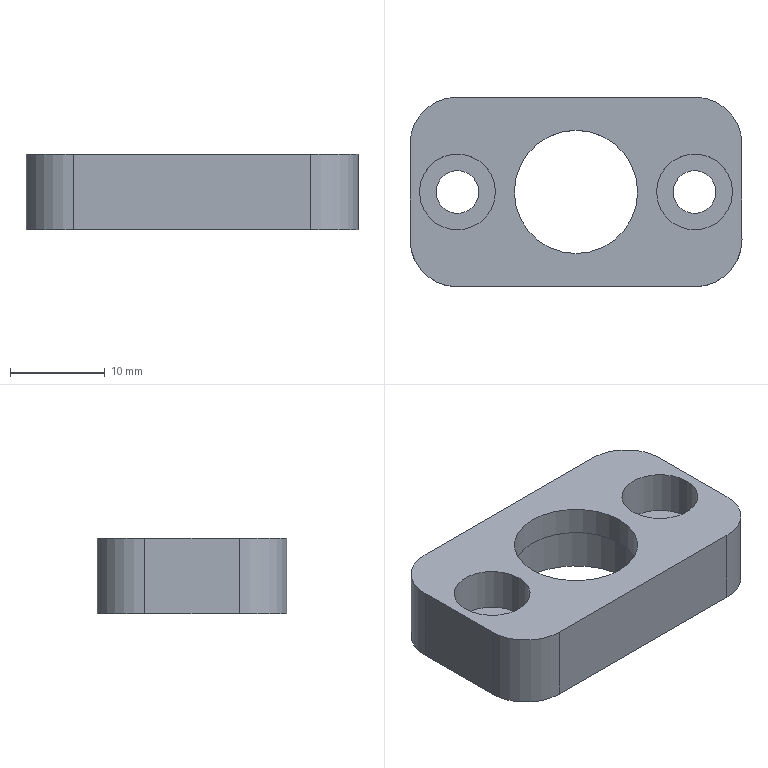Part | NX | 1 solid | 19 faces | box 35 x 20 x 8 mm | volume 3576 mm3 | cylinder 10 | plane 9 | commonest cylinder face diameters 10 x4 4.5 x2 8 x2 13 x1 15 x1
STEP:
#1=CARTESIAN_POINT('',(6.5,0.,8.));
#2=VERTEX_POINT('',#1);
#3=CARTESIAN_POINT('',(0.,0.,8.));
#4=DIRECTION('',(0.,0.,1.));
#5=DIRECTION('',(1.,0.,0.));
#6=AXIS2_PLACEMENT_3D('',#3,#4,#5);
#7=CIRCLE('',#6,6.5);
#8=EDGE_CURVE('',#2,#2,#7,.T.);
#9=ORIENTED_EDGE('',*,*,#8,.T.);
#10=EDGE_LOOP('',(#9));
#11=FACE_BOUND('',#10,.T.);
#12=CARTESIAN_POINT('',(-6.5,0.,5.));
#13=VERTEX_POINT('',#12);
#14=CARTESIAN_POINT('',(0.,0.,5.));
#15=DIRECTION('',(0.,0.,-1.));
#16=DIRECTION('',(-1.,0.,0.));
#17=AXIS2_PLACEMENT_3D('',#14,#15,#16);
#18=CIRCLE('',#17,6.5);
#19=EDGE_CURVE('',#13,#13,#18,.F.);
#20=ORIENTED_EDGE('',*,*,#19,.F.);
#21=EDGE_LOOP('',(#20));
#22=FACE_BOUND('',#21,.T.);
#23=CARTESIAN_POINT('',(0.,0.,0.));
#24=DIRECTION('',(0.,0.,1.));
#25=DIRECTION('',(1.,0.,0.));
#26=AXIS2_PLACEMENT_3D('',#23,#24,#25);
#27=CYLINDRICAL_SURFACE('',#26,6.5);
#28=ADVANCED_FACE('',(#11,#22),#27,.F.);
#29=CARTESIAN_POINT('',(17.5,-5.,8.));
#30=VERTEX_POINT('',#29);
#31=CARTESIAN_POINT('',(17.5,5.,8.));
#32=VERTEX_POINT('',#31);
#33=CARTESIAN_POINT('',(17.5,10.,8.));
#34=DIRECTION('',(0.,1.,0.));
#35=VECTOR('',#34,1000.);
#36=LINE('',#33,#35);
#37=EDGE_CURVE('',#30,#32,#36,.T.);
#38=ORIENTED_EDGE('',*,*,#37,.F.);
#39=CARTESIAN_POINT('',(17.5,-5.,0.));
#40=VERTEX_POINT('',#39);
#41=CARTESIAN_POINT('',(17.5,-5.,8.));
#42=DIRECTION('',(0.,0.,-1.));
#43=VECTOR('',#42,1000.);
#44=LINE('',#41,#43);
#45=EDGE_CURVE('',#30,#40,#44,.T.);
#46=ORIENTED_EDGE('',*,*,#45,.T.);
#47=CARTESIAN_POINT('',(17.5,5.,0.));
#48=VERTEX_POINT('',#47);
#49=CARTESIAN_POINT('',(17.5,10.,0.));
#50=DIRECTION('',(0.,1.,0.));
#51=VECTOR('',#50,1000.);
#52=LINE('',#49,#51);
#53=EDGE_CURVE('',#40,#48,#52,.T.);
#54=ORIENTED_EDGE('',*,*,#53,.T.);
#55=CARTESIAN_POINT('',(17.5,5.,8.));
#56=DIRECTION('',(0.,0.,-1.));
#57=VECTOR('',#56,1000.);
#58=LINE('',#55,#57);
#59=EDGE_CURVE('',#48,#32,#58,.F.);
#60=ORIENTED_EDGE('',*,*,#59,.T.);
#61=EDGE_LOOP('',(#38,#46,#54,#60));
#62=FACE_BOUND('',#61,.T.);
#63=CARTESIAN_POINT('',(17.5,10.,8.));
#64=DIRECTION('',(-1.,0.,0.));
#65=DIRECTION('',(0.,-1.,0.));
#66=AXIS2_PLACEMENT_3D('',#63,#64,#65);
#67=PLANE('',#66);
#68=ADVANCED_FACE('',(#62),#67,.F.);
#69=CARTESIAN_POINT('',(12.5,10.,0.));
#70=VERTEX_POINT('',#69);
#71=CARTESIAN_POINT('',(-12.5,10.,0.));
#72=VERTEX_POINT('',#71);
#73=CARTESIAN_POINT('',(-17.5,10.,0.));
#74=DIRECTION('',(-1.,0.,0.));
#75=VECTOR('',#74,1000.);
#76=LINE('',#73,#75);
#77=EDGE_CURVE('',#70,#72,#76,.T.);
#78=ORIENTED_EDGE('',*,*,#77,.T.);
#79=CARTESIAN_POINT('',(-12.5,10.,8.));
#80=VERTEX_POINT('',#79);
#81=CARTESIAN_POINT('',(-12.5,10.,8.));
#82=DIRECTION('',(0.,0.,-1.));
#83=VECTOR('',#82,1000.);
#84=LINE('',#81,#83);
#85=EDGE_CURVE('',#72,#80,#84,.F.);
#86=ORIENTED_EDGE('',*,*,#85,.T.);
#87=CARTESIAN_POINT('',(12.5,10.,8.));
#88=VERTEX_POINT('',#87);
#89=CARTESIAN_POINT('',(-17.5,10.,8.));
#90=DIRECTION('',(-1.,0.,0.));
#91=VECTOR('',#90,1000.);
#92=LINE('',#89,#91);
#93=EDGE_CURVE('',#88,#80,#92,.T.);
#94=ORIENTED_EDGE('',*,*,#93,.F.);
#95=CARTESIAN_POINT('',(12.5,10.,8.));
#96=DIRECTION('',(0.,0.,-1.));
#97=VECTOR('',#96,1000.);
#98=LINE('',#95,#97);
#99=EDGE_CURVE('',#88,#70,#98,.T.);
#100=ORIENTED_EDGE('',*,*,#99,.T.);
#101=EDGE_LOOP('',(#78,#86,#94,#100));
#102=FACE_BOUND('',#101,.T.);
#103=CARTESIAN_POINT('',(-17.5,10.,8.));
#104=DIRECTION('',(0.,-1.,0.));
#105=DIRECTION('',(0.,0.,-1.));
#106=AXIS2_PLACEMENT_3D('',#103,#104,#105);
#107=PLANE('',#106);
#108=ADVANCED_FACE('',(#102),#107,.F.);
#109=CARTESIAN_POINT('',(-17.5,5.,0.));
#110=VERTEX_POINT('',#109);
#111=CARTESIAN_POINT('',(-17.5,-5.,0.));
#112=VERTEX_POINT('',#111);
#113=CARTESIAN_POINT('',(-17.5,10.,0.));
#114=DIRECTION('',(0.,-1.,0.));
#115=VECTOR('',#114,1000.);
#116=LINE('',#113,#115);
#117=EDGE_CURVE('',#110,#112,#116,.T.);
#118=ORIENTED_EDGE('',*,*,#117,.T.);
#119=CARTESIAN_POINT('',(-17.5,-5.,8.));
#120=VERTEX_POINT('',#119);
#121=CARTESIAN_POINT('',(-17.5,-5.,8.));
#122=DIRECTION('',(0.,0.,-1.));
#123=VECTOR('',#122,1000.);
#124=LINE('',#121,#123);
#125=EDGE_CURVE('',#112,#120,#124,.F.);
#126=ORIENTED_EDGE('',*,*,#125,.T.);
#127=CARTESIAN_POINT('',(-17.5,5.,8.));
#128=VERTEX_POINT('',#127);
#129=CARTESIAN_POINT('',(-17.5,10.,8.));
#130=DIRECTION('',(0.,-1.,0.));
#131=VECTOR('',#130,1000.);
#132=LINE('',#129,#131);
#133=EDGE_CURVE('',#128,#120,#132,.T.);
#134=ORIENTED_EDGE('',*,*,#133,.F.);
#135=CARTESIAN_POINT('',(-17.5,5.,8.));
#136=DIRECTION('',(0.,0.,-1.));
#137=VECTOR('',#136,1000.);
#138=LINE('',#135,#137);
#139=EDGE_CURVE('',#128,#110,#138,.T.);
#140=ORIENTED_EDGE('',*,*,#139,.T.);
#141=EDGE_LOOP('',(#118,#126,#134,#140));
#142=FACE_BOUND('',#141,.T.);
#143=CARTESIAN_POINT('',(-17.5,10.,8.));
#144=DIRECTION('',(1.,0.,0.));
#145=DIRECTION('',(0.,1.,0.));
#146=AXIS2_PLACEMENT_3D('',#143,#144,#145);
#147=PLANE('',#146);
#148=ADVANCED_FACE('',(#142),#147,.F.);
#149=CARTESIAN_POINT('',(-12.5,-10.,0.));
#150=VERTEX_POINT('',#149);
#151=CARTESIAN_POINT('',(12.5,-10.,0.));
#152=VERTEX_POINT('',#151);
#153=CARTESIAN_POINT('',(-17.5,-10.,0.));
#154=DIRECTION('',(1.,0.,0.));
#155=VECTOR('',#154,1000.);
#156=LINE('',#153,#155);
#157=EDGE_CURVE('',#150,#152,#156,.T.);
#158=ORIENTED_EDGE('',*,*,#157,.T.);
#159=CARTESIAN_POINT('',(12.5,-10.,8.));
#160=VERTEX_POINT('',#159);
#161=CARTESIAN_POINT('',(12.5,-10.,8.));
#162=DIRECTION('',(0.,0.,-1.));
#163=VECTOR('',#162,1000.);
#164=LINE('',#161,#163);
#165=EDGE_CURVE('',#152,#160,#164,.F.);
#166=ORIENTED_EDGE('',*,*,#165,.T.);
#167=CARTESIAN_POINT('',(-12.5,-10.,8.));
#168=VERTEX_POINT('',#167);
#169=CARTESIAN_POINT('',(-17.5,-10.,8.));
#170=DIRECTION('',(1.,0.,0.));
#171=VECTOR('',#170,1000.);
#172=LINE('',#169,#171);
#173=EDGE_CURVE('',#168,#160,#172,.T.);
#174=ORIENTED_EDGE('',*,*,#173,.F.);
#175=CARTESIAN_POINT('',(-12.5,-10.,8.));
#176=DIRECTION('',(0.,0.,-1.));
#177=VECTOR('',#176,1000.);
#178=LINE('',#175,#177);
#179=EDGE_CURVE('',#168,#150,#178,.T.);
#180=ORIENTED_EDGE('',*,*,#179,.T.);
#181=EDGE_LOOP('',(#158,#166,#174,#180));
#182=FACE_BOUND('',#181,.T.);
#183=CARTESIAN_POINT('',(-17.5,-10.,8.));
#184=DIRECTION('',(0.,1.,0.));
#185=DIRECTION('',(0.,0.,1.));
#186=AXIS2_PLACEMENT_3D('',#183,#184,#185);
#187=PLANE('',#186);
#188=ADVANCED_FACE('',(#182),#187,.F.);
#189=CARTESIAN_POINT('',(-8.5,0.,8.));
#190=VERTEX_POINT('',#189);
#191=CARTESIAN_POINT('',(-12.5,0.,8.));
#192=DIRECTION('',(0.,0.,1.));
#193=DIRECTION('',(1.,0.,0.));
#194=AXIS2_PLACEMENT_3D('',#191,#192,#193);
#195=CIRCLE('',#194,4.);
#196=EDGE_CURVE('',#190,#190,#195,.T.);
#197=ORIENTED_EDGE('',*,*,#196,.F.);
#198=EDGE_LOOP('',(#197));
#199=FACE_BOUND('',#198,.T.);
#200=CARTESIAN_POINT('',(16.5,0.,8.));
#201=VERTEX_POINT('',#200);
#202=CARTESIAN_POINT('',(12.5,0.,8.));
#203=DIRECTION('',(0.,0.,1.));
#204=DIRECTION('',(1.,0.,0.));
#205=AXIS2_PLACEMENT_3D('',#202,#203,#204);
#206=CIRCLE('',#205,4.);
#207=EDGE_CURVE('',#201,#201,#206,.T.);
#208=ORIENTED_EDGE('',*,*,#207,.F.);
#209=EDGE_LOOP('',(#208));
#210=FACE_BOUND('',#209,.T.);
#211=ORIENTED_EDGE('',*,*,#8,.F.);
#212=EDGE_LOOP('',(#211));
#213=FACE_BOUND('',#212,.T.);
#214=ORIENTED_EDGE('',*,*,#173,.T.);
#215=CARTESIAN_POINT('',(12.5,-5.,8.));
#216=DIRECTION('',(0.,0.,1.));
#217=DIRECTION('',(1.,0.,0.));
#218=AXIS2_PLACEMENT_3D('',#215,#216,#217);
#219=CIRCLE('',#218,5.);
#220=EDGE_CURVE('',#160,#30,#219,.T.);
#221=ORIENTED_EDGE('',*,*,#220,.T.);
#222=ORIENTED_EDGE('',*,*,#37,.T.);
#223=CARTESIAN_POINT('',(12.5,5.,8.));
#224=DIRECTION('',(0.,0.,1.));
#225=DIRECTION('',(1.,0.,0.));
#226=AXIS2_PLACEMENT_3D('',#223,#224,#225);
#227=CIRCLE('',#226,5.);
#228=EDGE_CURVE('',#32,#88,#227,.T.);
#229=ORIENTED_EDGE('',*,*,#228,.T.);
#230=ORIENTED_EDGE('',*,*,#93,.T.);
#231=CARTESIAN_POINT('',(-12.5,5.,8.));
#232=DIRECTION('',(0.,0.,1.));
#233=DIRECTION('',(1.,0.,0.));
#234=AXIS2_PLACEMENT_3D('',#231,#232,#233);
#235=CIRCLE('',#234,5.);
#236=EDGE_CURVE('',#80,#128,#235,.T.);
#237=ORIENTED_EDGE('',*,*,#236,.T.);
#238=ORIENTED_EDGE('',*,*,#133,.T.);
#239=CARTESIAN_POINT('',(-12.5,-5.,8.));
#240=DIRECTION('',(0.,0.,1.));
#241=DIRECTION('',(1.,0.,0.));
#242=AXIS2_PLACEMENT_3D('',#239,#240,#241);
#243=CIRCLE('',#242,5.);
#244=EDGE_CURVE('',#120,#168,#243,.T.);
#245=ORIENTED_EDGE('',*,*,#244,.T.);
#246=EDGE_LOOP('',(#214,#221,#222,#229,#230,#237,#238,#245));
#247=FACE_BOUND('',#246,.T.);
#248=CARTESIAN_POINT('',(0.,0.,8.));
#249=DIRECTION('',(0.,0.,1.));
#250=DIRECTION('',(1.,0.,0.));
#251=AXIS2_PLACEMENT_3D('',#248,#249,#250);
#252=PLANE('',#251);
#253=ADVANCED_FACE('',(#199,#210,#213,#247),#252,.T.);
#254=CARTESIAN_POINT('',(-7.5,0.,0.));
#255=VERTEX_POINT('',#254);
#256=CARTESIAN_POINT('',(0.,0.,0.));
#257=DIRECTION('',(0.,0.,-1.));
#258=DIRECTION('',(-1.,0.,0.));
#259=AXIS2_PLACEMENT_3D('',#256,#257,#258);
#260=CIRCLE('',#259,7.5);
#261=EDGE_CURVE('',#255,#255,#260,.T.);
#262=ORIENTED_EDGE('',*,*,#261,.F.);
#263=EDGE_LOOP('',(#262));
#264=FACE_BOUND('',#263,.T.);
#265=CARTESIAN_POINT('',(-10.25,0.,0.));
#266=VERTEX_POINT('',#265);
#267=CARTESIAN_POINT('',(-12.5,0.,0.));
#268=DIRECTION('',(0.,0.,1.));
#269=DIRECTION('',(1.,0.,0.));
#270=AXIS2_PLACEMENT_3D('',#267,#268,#269);
#271=CIRCLE('',#270,2.25);
#272=EDGE_CURVE('',#266,#266,#271,.T.);
#273=ORIENTED_EDGE('',*,*,#272,.T.);
#274=EDGE_LOOP('',(#273));
#275=FACE_BOUND('',#274,.T.);
#276=CARTESIAN_POINT('',(14.75,0.,0.));
#277=VERTEX_POINT('',#276);
#278=CARTESIAN_POINT('',(12.5,0.,0.));
#279=DIRECTION('',(0.,0.,1.));
#280=DIRECTION('',(1.,0.,0.));
#281=AXIS2_PLACEMENT_3D('',#278,#279,#280);
#282=CIRCLE('',#281,2.25);
#283=EDGE_CURVE('',#277,#277,#282,.T.);
#284=ORIENTED_EDGE('',*,*,#283,.T.);
#285=EDGE_LOOP('',(#284));
#286=FACE_BOUND('',#285,.T.);
#287=ORIENTED_EDGE('',*,*,#53,.F.);
#288=CARTESIAN_POINT('',(12.5,-5.,0.));
#289=DIRECTION('',(0.,0.,1.));
#290=DIRECTION('',(1.,0.,0.));
#291=AXIS2_PLACEMENT_3D('',#288,#289,#290);
#292=CIRCLE('',#291,5.);
#293=EDGE_CURVE('',#40,#152,#292,.F.);
#294=ORIENTED_EDGE('',*,*,#293,.T.);
#295=ORIENTED_EDGE('',*,*,#157,.F.);
#296=CARTESIAN_POINT('',(-12.5,-5.,0.));
#297=DIRECTION('',(0.,0.,1.));
#298=DIRECTION('',(1.,0.,0.));
#299=AXIS2_PLACEMENT_3D('',#296,#297,#298);
#300=CIRCLE('',#299,5.);
#301=EDGE_CURVE('',#150,#112,#300,.F.);
#302=ORIENTED_EDGE('',*,*,#301,.T.);
#303=ORIENTED_EDGE('',*,*,#117,.F.);
#304=CARTESIAN_POINT('',(-12.5,5.,0.));
#305=DIRECTION('',(0.,0.,1.));
#306=DIRECTION('',(1.,0.,0.));
#307=AXIS2_PLACEMENT_3D('',#304,#305,#306);
#308=CIRCLE('',#307,5.);
#309=EDGE_CURVE('',#110,#72,#308,.F.);
#310=ORIENTED_EDGE('',*,*,#309,.T.);
#311=ORIENTED_EDGE('',*,*,#77,.F.);
#312=CARTESIAN_POINT('',(12.5,5.,0.));
#313=DIRECTION('',(0.,0.,1.));
#314=DIRECTION('',(1.,0.,0.));
#315=AXIS2_PLACEMENT_3D('',#312,#313,#314);
#316=CIRCLE('',#315,5.);
#317=EDGE_CURVE('',#70,#48,#316,.F.);
#318=ORIENTED_EDGE('',*,*,#317,.T.);
#319=EDGE_LOOP('',(#287,#294,#295,#302,#303,#310,#311,#318));
#320=FACE_BOUND('',#319,.T.);
#321=CARTESIAN_POINT('',(0.,0.,0.));
#322=DIRECTION('',(0.,0.,1.));
#323=DIRECTION('',(1.,0.,0.));
#324=AXIS2_PLACEMENT_3D('',#321,#322,#323);
#325=PLANE('',#324);
#326=ADVANCED_FACE('',(#264,#275,#286,#320),#325,.F.);
#327=ORIENTED_EDGE('',*,*,#220,.F.);
#328=ORIENTED_EDGE('',*,*,#165,.F.);
#329=ORIENTED_EDGE('',*,*,#293,.F.);
#330=ORIENTED_EDGE('',*,*,#45,.F.);
#331=EDGE_LOOP('',(#327,#328,#329,#330));
#332=FACE_BOUND('',#331,.T.);
#333=CARTESIAN_POINT('',(12.5,-5.,8.));
#334=DIRECTION('',(0.,0.,-1.));
#335=DIRECTION('',(-1.,0.,0.));
#336=AXIS2_PLACEMENT_3D('',#333,#334,#335);
#337=CYLINDRICAL_SURFACE('',#336,5.);
#338=ADVANCED_FACE('',(#332),#337,.T.);
#339=ORIENTED_EDGE('',*,*,#244,.F.);
#340=ORIENTED_EDGE('',*,*,#125,.F.);
#341=ORIENTED_EDGE('',*,*,#301,.F.);
#342=ORIENTED_EDGE('',*,*,#179,.F.);
#343=EDGE_LOOP('',(#339,#340,#341,#342));
#344=FACE_BOUND('',#343,.T.);
#345=CARTESIAN_POINT('',(-12.5,-5.,8.));
#346=DIRECTION('',(0.,0.,-1.));
#347=DIRECTION('',(-1.,0.,0.));
#348=AXIS2_PLACEMENT_3D('',#345,#346,#347);
#349=CYLINDRICAL_SURFACE('',#348,5.);
#350=ADVANCED_FACE('',(#344),#349,.T.);
#351=ORIENTED_EDGE('',*,*,#236,.F.);
#352=ORIENTED_EDGE('',*,*,#85,.F.);
#353=ORIENTED_EDGE('',*,*,#309,.F.);
#354=ORIENTED_EDGE('',*,*,#139,.F.);
#355=EDGE_LOOP('',(#351,#352,#353,#354));
#356=FACE_BOUND('',#355,.T.);
#357=CARTESIAN_POINT('',(-12.5,5.,8.));
#358=DIRECTION('',(0.,0.,-1.));
#359=DIRECTION('',(-1.,0.,0.));
#360=AXIS2_PLACEMENT_3D('',#357,#358,#359);
#361=CYLINDRICAL_SURFACE('',#360,5.);
#362=ADVANCED_FACE('',(#356),#361,.T.);
#363=ORIENTED_EDGE('',*,*,#228,.F.);
#364=ORIENTED_EDGE('',*,*,#59,.F.);
#365=ORIENTED_EDGE('',*,*,#317,.F.);
#366=ORIENTED_EDGE('',*,*,#99,.F.);
#367=EDGE_LOOP('',(#363,#364,#365,#366));
#368=FACE_BOUND('',#367,.T.);
#369=CARTESIAN_POINT('',(12.5,5.,8.));
#370=DIRECTION('',(0.,0.,-1.));
#371=DIRECTION('',(-1.,0.,0.));
#372=AXIS2_PLACEMENT_3D('',#369,#370,#371);
#373=CYLINDRICAL_SURFACE('',#372,5.);
#374=ADVANCED_FACE('',(#368),#373,.T.);
#375=ORIENTED_EDGE('',*,*,#283,.F.);
#376=EDGE_LOOP('',(#375));
#377=FACE_BOUND('',#376,.T.);
#378=CARTESIAN_POINT('',(14.75,0.,3.4));
#379=VERTEX_POINT('',#378);
#380=CARTESIAN_POINT('',(12.5,0.,3.4));
#381=DIRECTION('',(0.,0.,1.));
#382=DIRECTION('',(1.,0.,0.));
#383=AXIS2_PLACEMENT_3D('',#380,#381,#382);
#384=CIRCLE('',#383,2.25);
#385=EDGE_CURVE('',#379,#379,#384,.T.);
#386=ORIENTED_EDGE('',*,*,#385,.T.);
#387=EDGE_LOOP('',(#386));
#388=FACE_BOUND('',#387,.T.);
#389=CARTESIAN_POINT('',(12.5,0.,8.));
#390=DIRECTION('',(0.,0.,1.));
#391=DIRECTION('',(1.,0.,0.));
#392=AXIS2_PLACEMENT_3D('',#389,#390,#391);
#393=CYLINDRICAL_SURFACE('',#392,2.25);
#394=ADVANCED_FACE('',(#377,#388),#393,.F.);
#395=ORIENTED_EDGE('',*,*,#385,.F.);
#396=EDGE_LOOP('',(#395));
#397=FACE_BOUND('',#396,.T.);
#398=CARTESIAN_POINT('',(16.5,0.,3.4));
#399=VERTEX_POINT('',#398);
#400=CARTESIAN_POINT('',(12.5,0.,3.4));
#401=DIRECTION('',(0.,0.,1.));
#402=DIRECTION('',(1.,0.,0.));
#403=AXIS2_PLACEMENT_3D('',#400,#401,#402);
#404=CIRCLE('',#403,4.);
#405=EDGE_CURVE('',#399,#399,#404,.T.);
#406=ORIENTED_EDGE('',*,*,#405,.T.);
#407=EDGE_LOOP('',(#406));
#408=FACE_BOUND('',#407,.T.);
#409=CARTESIAN_POINT('',(14.75,0.,3.4));
#410=DIRECTION('',(0.,0.,-1.));
#411=DIRECTION('',(-1.,0.,0.));
#412=AXIS2_PLACEMENT_3D('',#409,#410,#411);
#413=PLANE('',#412);
#414=ADVANCED_FACE('',(#397,#408),#413,.F.);
#415=ORIENTED_EDGE('',*,*,#405,.F.);
#416=EDGE_LOOP('',(#415));
#417=FACE_BOUND('',#416,.T.);
#418=ORIENTED_EDGE('',*,*,#207,.T.);
#419=EDGE_LOOP('',(#418));
#420=FACE_BOUND('',#419,.T.);
#421=CARTESIAN_POINT('',(12.5,0.,8.));
#422=DIRECTION('',(0.,0.,1.));
#423=DIRECTION('',(1.,0.,0.));
#424=AXIS2_PLACEMENT_3D('',#421,#422,#423);
#425=CYLINDRICAL_SURFACE('',#424,4.);
#426=ADVANCED_FACE('',(#417,#420),#425,.F.);
#427=ORIENTED_EDGE('',*,*,#272,.F.);
#428=EDGE_LOOP('',(#427));
#429=FACE_BOUND('',#428,.T.);
#430=CARTESIAN_POINT('',(-10.25,0.,3.4));
#431=VERTEX_POINT('',#430);
#432=CARTESIAN_POINT('',(-12.5,0.,3.4));
#433=DIRECTION('',(0.,0.,1.));
#434=DIRECTION('',(1.,0.,0.));
#435=AXIS2_PLACEMENT_3D('',#432,#433,#434);
#436=CIRCLE('',#435,2.25);
#437=EDGE_CURVE('',#431,#431,#436,.T.);
#438=ORIENTED_EDGE('',*,*,#437,.T.);
#439=EDGE_LOOP('',(#438));
#440=FACE_BOUND('',#439,.T.);
#441=CARTESIAN_POINT('',(-12.5,0.,8.));
#442=DIRECTION('',(0.,0.,1.));
#443=DIRECTION('',(1.,0.,0.));
#444=AXIS2_PLACEMENT_3D('',#441,#442,#443);
#445=CYLINDRICAL_SURFACE('',#444,2.25);
#446=ADVANCED_FACE('',(#429,#440),#445,.F.);
#447=ORIENTED_EDGE('',*,*,#437,.F.);
#448=EDGE_LOOP('',(#447));
#449=FACE_BOUND('',#448,.T.);
#450=CARTESIAN_POINT('',(-8.5,0.,3.4));
#451=VERTEX_POINT('',#450);
#452=CARTESIAN_POINT('',(-12.5,0.,3.4));
#453=DIRECTION('',(0.,0.,1.));
#454=DIRECTION('',(1.,0.,0.));
#455=AXIS2_PLACEMENT_3D('',#452,#453,#454);
#456=CIRCLE('',#455,4.);
#457=EDGE_CURVE('',#451,#451,#456,.T.);
#458=ORIENTED_EDGE('',*,*,#457,.T.);
#459=EDGE_LOOP('',(#458));
#460=FACE_BOUND('',#459,.T.);
#461=CARTESIAN_POINT('',(-10.25,0.,3.4));
#462=DIRECTION('',(0.,0.,-1.));
#463=DIRECTION('',(-1.,0.,0.));
#464=AXIS2_PLACEMENT_3D('',#461,#462,#463);
#465=PLANE('',#464);
#466=ADVANCED_FACE('',(#449,#460),#465,.F.);
#467=ORIENTED_EDGE('',*,*,#457,.F.);
#468=EDGE_LOOP('',(#467));
#469=FACE_BOUND('',#468,.T.);
#470=ORIENTED_EDGE('',*,*,#196,.T.);
#471=EDGE_LOOP('',(#470));
#472=FACE_BOUND('',#471,.T.);
#473=CARTESIAN_POINT('',(-12.5,0.,8.));
#474=DIRECTION('',(0.,0.,1.));
#475=DIRECTION('',(1.,0.,0.));
#476=AXIS2_PLACEMENT_3D('',#473,#474,#475);
#477=CYLINDRICAL_SURFACE('',#476,4.);
#478=ADVANCED_FACE('',(#469,#472),#477,.F.);
#479=CARTESIAN_POINT('',(-7.5,0.,5.));
#480=VERTEX_POINT('',#479);
#481=CARTESIAN_POINT('',(0.,0.,5.));
#482=DIRECTION('',(0.,0.,-1.));
#483=DIRECTION('',(-1.,0.,0.));
#484=AXIS2_PLACEMENT_3D('',#481,#482,#483);
#485=CIRCLE('',#484,7.5);
#486=EDGE_CURVE('',#480,#480,#485,.T.);
#487=ORIENTED_EDGE('',*,*,#486,.T.);
#488=EDGE_LOOP('',(#487));
#489=FACE_BOUND('',#488,.T.);
#490=ORIENTED_EDGE('',*,*,#19,.T.);
#491=EDGE_LOOP('',(#490));
#492=FACE_BOUND('',#491,.T.);
#493=CARTESIAN_POINT('',(0.,0.,5.));
#494=DIRECTION('',(0.,0.,-1.));
#495=DIRECTION('',(-1.,0.,0.));
#496=AXIS2_PLACEMENT_3D('',#493,#494,#495);
#497=PLANE('',#496);
#498=ADVANCED_FACE('',(#489,#492),#497,.T.);
#499=ORIENTED_EDGE('',*,*,#486,.F.);
#500=EDGE_LOOP('',(#499));
#501=FACE_BOUND('',#500,.T.);
#502=ORIENTED_EDGE('',*,*,#261,.T.);
#503=EDGE_LOOP('',(#502));
#504=FACE_BOUND('',#503,.T.);
#505=CARTESIAN_POINT('',(0.,0.,5.));
#506=DIRECTION('',(0.,0.,-1.));
#507=DIRECTION('',(-1.,0.,0.));
#508=AXIS2_PLACEMENT_3D('',#505,#506,#507);
#509=CYLINDRICAL_SURFACE('',#508,7.5);
#510=ADVANCED_FACE('',(#501,#504),#509,.F.);
#511=CLOSED_SHELL('',(#28,#68,#108,#148,#188,#253,#326,#338,#350,#362,#374,#394,#414,#426,#446,#466,#478,#498,#510));
#512=MANIFOLD_SOLID_BREP('',#511);
#513=(LENGTH_UNIT()NAMED_UNIT(*)SI_UNIT(.MILLI.,.METRE.));
#514=UNCERTAINTY_MEASURE_WITH_UNIT(LENGTH_MEASURE(0.00001),#513,'','');
#515=(NAMED_UNIT(*)PLANE_ANGLE_UNIT()SI_UNIT($,.RADIAN.));
#516=(NAMED_UNIT(*)SI_UNIT($,.STERADIAN.)SOLID_ANGLE_UNIT());
#517=(GEOMETRIC_REPRESENTATION_CONTEXT(3)GLOBAL_UNCERTAINTY_ASSIGNED_CONTEXT((#514))GLOBAL_UNIT_ASSIGNED_CONTEXT((#513,#515,#516))REPRESENTATION_CONTEXT('',''));
#518=ADVANCED_BREP_SHAPE_REPRESENTATION('',(#512),#517);